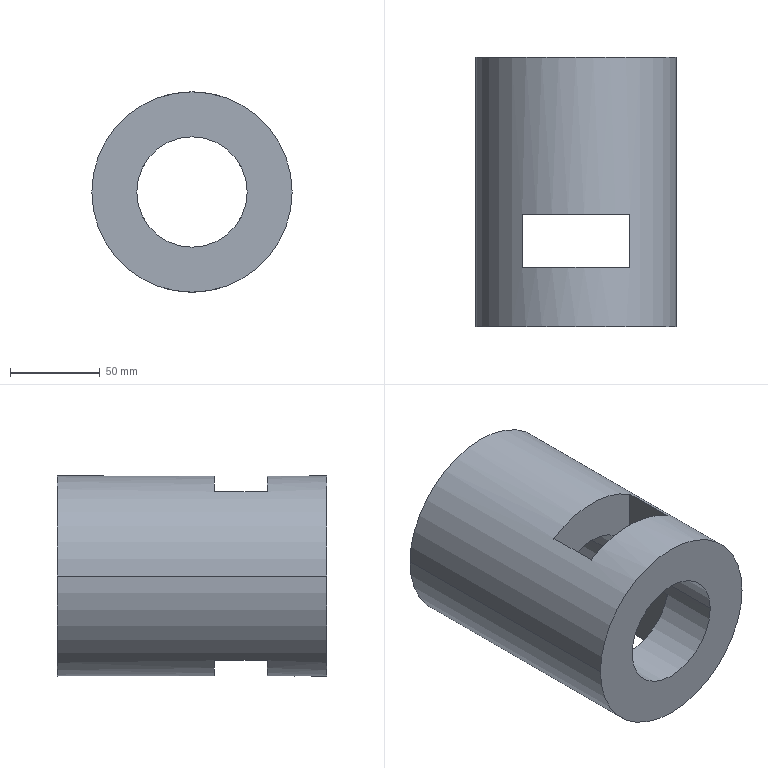Part | STEP file | Input 1-5 | 1 solid | 17 faces | box 111.5 x 150 x 111.5 mm | volume 917688 mm3 | plane 11 | cylinder 6 | commonest cylinder face diameters 10 x2 61.5 x2 111.5 x2
STEP:
#1=CARTESIAN_POINT('',(-753.859,1587.424,3132.342));
#2=VERTEX_POINT('',#1);
#3=CARTESIAN_POINT('',(-743.859,1587.424,3132.342));
#4=VERTEX_POINT('',#3);
#5=CARTESIAN_POINT('',(-748.859,1587.424,3132.342));
#6=DIRECTION('',(0.,0.,-1.));
#7=DIRECTION('',(1.,0.,0.));
#8=AXIS2_PLACEMENT_3D('',#5,#6,#7);
#9=CIRCLE('',#8,5.);
#10=EDGE_CURVE('',#2,#4,#9,.T.);
#11=ORIENTED_EDGE('',*,*,#10,.F.);
#12=CARTESIAN_POINT('',(-753.859,1587.424,3116.816));
#13=VERTEX_POINT('',#12);
#14=CARTESIAN_POINT('',(-753.859,1587.424,3132.342));
#15=DIRECTION('',(0.,0.,1.));
#16=VECTOR('',#15,1000.);
#17=LINE('',#14,#16);
#18=EDGE_CURVE('',#13,#2,#17,.T.);
#19=ORIENTED_EDGE('',*,*,#18,.F.);
#20=CARTESIAN_POINT('',(-743.859,1587.424,3116.816));
#21=VERTEX_POINT('',#20);
#22=CARTESIAN_POINT('',(-743.859,1587.424,3116.816));
#23=CARTESIAN_POINT('',(-743.859,1587.754,3116.816));
#24=CARTESIAN_POINT('',(-743.891,1588.079,3116.813));
#25=CARTESIAN_POINT('',(-743.987,1588.558,3116.805));
#26=CARTESIAN_POINT('',(-744.026,1588.717,3116.802));
#27=CARTESIAN_POINT('',(-744.121,1589.031,3116.793));
#28=CARTESIAN_POINT('',(-744.177,1589.187,3116.789));
#29=CARTESIAN_POINT('',(-744.365,1589.641,3116.773));
#30=CARTESIAN_POINT('',(-744.519,1589.928,3116.761));
#31=CARTESIAN_POINT('',(-744.882,1590.472,3116.733));
#32=CARTESIAN_POINT('',(-745.093,1590.729,3116.719));
#33=CARTESIAN_POINT('',(-745.554,1591.19,3116.689));
#34=CARTESIAN_POINT('',(-745.805,1591.397,3116.675));
#35=CARTESIAN_POINT('',(-746.352,1591.762,3116.647));
#36=CARTESIAN_POINT('',(-746.643,1591.917,3116.635));
#37=CARTESIAN_POINT('',(-747.244,1592.167,3116.614));
#38=CARTESIAN_POINT('',(-747.559,1592.263,3116.606));
#39=CARTESIAN_POINT('',(-748.205,1592.391,3116.595));
#40=CARTESIAN_POINT('',(-748.529,1592.423,3116.592));
#41=CARTESIAN_POINT('',(-749.182,1592.424,3116.592));
#42=CARTESIAN_POINT('',(-749.513,1592.391,3116.595));
#43=CARTESIAN_POINT('',(-750.154,1592.264,3116.606));
#44=CARTESIAN_POINT('',(-750.466,1592.17,3116.614));
#45=CARTESIAN_POINT('',(-750.92,1591.982,3116.63));
#46=CARTESIAN_POINT('',(-751.07,1591.911,3116.635));
#47=CARTESIAN_POINT('',(-751.36,1591.756,3116.648));
#48=CARTESIAN_POINT('',(-751.5,1591.672,3116.654));
#49=CARTESIAN_POINT('',(-751.906,1591.401,3116.674));
#50=CARTESIAN_POINT('',(-752.158,1591.195,3116.689));
#51=CARTESIAN_POINT('',(-752.625,1590.728,3116.719));
#52=CARTESIAN_POINT('',(-752.832,1590.476,3116.733));
#53=CARTESIAN_POINT('',(-753.104,1590.07,3116.754));
#54=CARTESIAN_POINT('',(-753.188,1589.93,3116.76));
#55=CARTESIAN_POINT('',(-753.343,1589.641,3116.772));
#56=CARTESIAN_POINT('',(-753.414,1589.491,3116.778));
#57=CARTESIAN_POINT('',(-753.603,1589.037,3116.794));
#58=CARTESIAN_POINT('',(-753.697,1588.726,3116.802));
#59=CARTESIAN_POINT('',(-753.826,1588.085,3116.813));
#60=CARTESIAN_POINT('',(-753.859,1587.754,3116.816));
#61=CARTESIAN_POINT('',(-753.859,1587.424,3116.816));
#62=B_SPLINE_CURVE_WITH_KNOTS('',3,(#22,#23,#24,#25,#26,#27,#28,#29,#30,#31,#32,#33,#34,#35,#36,#37,#38,#39,#40,#41,#42,#43,#44,#45,#46,#47,#48,#49,#50,#51,#52,#53,#54,#55,#56,#57,#58,#59,#60,#61),.UNSPECIFIED.,.F.,.F.,(4,2,2,2,2,2,2,2,2,2,2,2,2,2,2,2,2,2,2,4),(0.,0.0009773,0.001466,0.001955,0.002932,0.003909,0.004886,0.005864,0.006841,0.007818,0.008796,0.009773,0.01026,0.01075,0.01173,0.0127,0.01319,0.01368,0.01466,0.01564),.UNSPECIFIED.);
#63=EDGE_CURVE('',#21,#13,#62,.T.);
#64=ORIENTED_EDGE('',*,*,#63,.F.);
#65=CARTESIAN_POINT('',(-743.859,1587.424,3132.342));
#66=DIRECTION('',(0.,0.,1.));
#67=VECTOR('',#66,1000.);
#68=LINE('',#65,#67);
#69=EDGE_CURVE('',#21,#4,#68,.T.);
#70=ORIENTED_EDGE('',*,*,#69,.T.);
#71=EDGE_LOOP('',(#11,#19,#64,#70));
#72=FACE_OUTER_BOUND('',#71,.T.);
#73=CARTESIAN_POINT('',(-748.859,1587.424,3132.342));
#74=DIRECTION('',(0.,0.,-1.));
#75=DIRECTION('',(-1.,0.,0.));
#76=AXIS2_PLACEMENT_3D('',#73,#74,#75);
#77=CYLINDRICAL_SURFACE('',#76,5.);
#78=ADVANCED_FACE('',(#72),#77,.F.);
#79=CARTESIAN_POINT('',(-718.859,1636.918,3179.092));
#80=VERTEX_POINT('',#79);
#81=CARTESIAN_POINT('',(-718.859,1607.418,3179.092));
#82=VERTEX_POINT('',#81);
#83=CARTESIAN_POINT('',(-718.859,1574.418,3179.092));
#84=DIRECTION('',(0.,-1.,0.));
#85=VECTOR('',#84,1000.);
#86=LINE('',#83,#85);
#87=EDGE_CURVE('',#80,#82,#86,.T.);
#88=ORIENTED_EDGE('',*,*,#87,.F.);
#89=CARTESIAN_POINT('',(-778.859,1636.918,3179.092));
#90=VERTEX_POINT('',#89);
#91=CARTESIAN_POINT('',(-748.859,1636.918,3172.342));
#92=DIRECTION('',(0.,1.,0.));
#93=DIRECTION('',(1.,0.,0.));
#94=AXIS2_PLACEMENT_3D('',#91,#92,#93);
#95=CIRCLE('',#94,30.75);
#96=EDGE_CURVE('',#90,#80,#95,.T.);
#97=ORIENTED_EDGE('',*,*,#96,.F.);
#98=CARTESIAN_POINT('',(-778.859,1607.418,3179.092));
#99=VERTEX_POINT('',#98);
#100=CARTESIAN_POINT('',(-778.859,1574.418,3179.092));
#101=DIRECTION('',(0.,1.,0.));
#102=VECTOR('',#101,1000.);
#103=LINE('',#100,#102);
#104=EDGE_CURVE('',#99,#90,#103,.T.);
#105=ORIENTED_EDGE('',*,*,#104,.F.);
#106=CARTESIAN_POINT('',(-748.859,1607.418,3172.342));
#107=DIRECTION('',(0.,-1.,0.));
#108=DIRECTION('',(-1.,0.,0.));
#109=AXIS2_PLACEMENT_3D('',#106,#107,#108);
#110=CIRCLE('',#109,30.75);
#111=EDGE_CURVE('',#82,#99,#110,.T.);
#112=ORIENTED_EDGE('',*,*,#111,.F.);
#113=EDGE_LOOP('',(#88,#97,#105,#112));
#114=FACE_BOUND('',#113,.T.);
#115=CARTESIAN_POINT('',(-718.109,1574.418,3172.342));
#116=VERTEX_POINT('',#115);
#117=CARTESIAN_POINT('',(-779.609,1574.418,3172.342));
#118=VERTEX_POINT('',#117);
#119=CARTESIAN_POINT('',(-748.859,1574.418,3172.342));
#120=DIRECTION('',(0.,-1.,0.));
#121=DIRECTION('',(-1.,0.,0.));
#122=AXIS2_PLACEMENT_3D('',#119,#120,#121);
#123=CIRCLE('',#122,30.75);
#124=EDGE_CURVE('',#116,#118,#123,.T.);
#125=ORIENTED_EDGE('',*,*,#124,.T.);
#126=CARTESIAN_POINT('',(-779.609,1724.418,3172.342));
#127=VERTEX_POINT('',#126);
#128=CARTESIAN_POINT('',(-779.609,1574.418,3172.342));
#129=DIRECTION('',(0.,-1.,0.));
#130=VECTOR('',#129,1000.);
#131=LINE('',#128,#130);
#132=EDGE_CURVE('',#127,#118,#131,.T.);
#133=ORIENTED_EDGE('',*,*,#132,.F.);
#134=CARTESIAN_POINT('',(-718.109,1724.418,3172.342));
#135=VERTEX_POINT('',#134);
#136=CARTESIAN_POINT('',(-748.859,1724.418,3172.342));
#137=DIRECTION('',(0.,-1.,0.));
#138=DIRECTION('',(-1.,0.,0.));
#139=AXIS2_PLACEMENT_3D('',#136,#137,#138);
#140=CIRCLE('',#139,30.75);
#141=EDGE_CURVE('',#135,#127,#140,.T.);
#142=ORIENTED_EDGE('',*,*,#141,.F.);
#143=CARTESIAN_POINT('',(-718.109,1574.418,3172.342));
#144=DIRECTION('',(0.,-1.,0.));
#145=VECTOR('',#144,1000.);
#146=LINE('',#143,#145);
#147=EDGE_CURVE('',#135,#116,#146,.T.);
#148=ORIENTED_EDGE('',*,*,#147,.T.);
#149=EDGE_LOOP('',(#125,#133,#142,#148));
#150=FACE_OUTER_BOUND('',#149,.T.);
#151=CARTESIAN_POINT('',(-748.859,1574.418,3172.342));
#152=DIRECTION('',(0.,1.,0.));
#153=DIRECTION('',(-1.,0.,0.));
#154=AXIS2_PLACEMENT_3D('',#151,#152,#153);
#155=CYLINDRICAL_SURFACE('',#154,30.75);
#156=ADVANCED_FACE('',(#114,#150),#155,.F.);
#157=CARTESIAN_POINT('',(-778.859,1607.418,3125.352));
#158=VERTEX_POINT('',#157);
#159=CARTESIAN_POINT('',(-718.859,1607.418,3125.352));
#160=VERTEX_POINT('',#159);
#161=CARTESIAN_POINT('',(-748.859,1607.418,3172.342));
#162=DIRECTION('',(0.,-1.,0.));
#163=DIRECTION('',(-1.,0.,0.));
#164=AXIS2_PLACEMENT_3D('',#161,#162,#163);
#165=CIRCLE('',#164,55.75);
#166=EDGE_CURVE('',#158,#160,#165,.T.);
#167=ORIENTED_EDGE('',*,*,#166,.T.);
#168=CARTESIAN_POINT('',(-718.859,1636.918,3125.352));
#169=VERTEX_POINT('',#168);
#170=CARTESIAN_POINT('',(-718.859,1574.418,3125.352));
#171=DIRECTION('',(0.,1.,0.));
#172=VECTOR('',#171,1000.);
#173=LINE('',#170,#172);
#174=EDGE_CURVE('',#160,#169,#173,.T.);
#175=ORIENTED_EDGE('',*,*,#174,.T.);
#176=CARTESIAN_POINT('',(-778.859,1636.918,3125.352));
#177=VERTEX_POINT('',#176);
#178=CARTESIAN_POINT('',(-748.859,1636.918,3172.342));
#179=DIRECTION('',(0.,1.,0.));
#180=DIRECTION('',(1.,0.,0.));
#181=AXIS2_PLACEMENT_3D('',#178,#179,#180);
#182=CIRCLE('',#181,55.75);
#183=EDGE_CURVE('',#169,#177,#182,.T.);
#184=ORIENTED_EDGE('',*,*,#183,.T.);
#185=CARTESIAN_POINT('',(-778.859,1574.418,3125.352));
#186=DIRECTION('',(0.,-1.,0.));
#187=VECTOR('',#186,1000.);
#188=LINE('',#185,#187);
#189=EDGE_CURVE('',#177,#158,#188,.T.);
#190=ORIENTED_EDGE('',*,*,#189,.T.);
#191=EDGE_LOOP('',(#167,#175,#184,#190));
#192=FACE_BOUND('',#191,.T.);
#193=ORIENTED_EDGE('',*,*,#63,.T.);
#194=CARTESIAN_POINT('',(-753.859,1587.424,3116.816));
#195=CARTESIAN_POINT('',(-753.859,1587.093,3116.816));
#196=CARTESIAN_POINT('',(-753.826,1586.768,3116.813));
#197=CARTESIAN_POINT('',(-753.731,1586.289,3116.805));
#198=CARTESIAN_POINT('',(-753.691,1586.13,3116.802));
#199=CARTESIAN_POINT('',(-753.596,1585.816,3116.793));
#200=CARTESIAN_POINT('',(-753.54,1585.66,3116.789));
#201=CARTESIAN_POINT('',(-753.352,1585.206,3116.773));
#202=CARTESIAN_POINT('',(-753.199,1584.919,3116.761));
#203=CARTESIAN_POINT('',(-752.836,1584.376,3116.733));
#204=CARTESIAN_POINT('',(-752.625,1584.118,3116.719));
#205=CARTESIAN_POINT('',(-752.164,1583.657,3116.689));
#206=CARTESIAN_POINT('',(-751.912,1583.451,3116.675));
#207=CARTESIAN_POINT('',(-751.366,1583.085,3116.647));
#208=CARTESIAN_POINT('',(-751.075,1582.93,3116.635));
#209=CARTESIAN_POINT('',(-750.474,1582.68,3116.614));
#210=CARTESIAN_POINT('',(-750.158,1582.584,3116.606));
#211=CARTESIAN_POINT('',(-749.513,1582.456,3116.595));
#212=CARTESIAN_POINT('',(-749.189,1582.424,3116.592));
#213=CARTESIAN_POINT('',(-748.536,1582.423,3116.592));
#214=CARTESIAN_POINT('',(-748.205,1582.456,3116.595));
#215=CARTESIAN_POINT('',(-747.563,1582.583,3116.606));
#216=CARTESIAN_POINT('',(-747.252,1582.678,3116.614));
#217=CARTESIAN_POINT('',(-746.797,1582.865,3116.63));
#218=CARTESIAN_POINT('',(-746.648,1582.936,3116.635));
#219=CARTESIAN_POINT('',(-746.358,1583.091,3116.648));
#220=CARTESIAN_POINT('',(-746.218,1583.175,3116.654));
#221=CARTESIAN_POINT('',(-745.812,1583.446,3116.674));
#222=CARTESIAN_POINT('',(-745.559,1583.652,3116.689));
#223=CARTESIAN_POINT('',(-745.092,1584.119,3116.719));
#224=CARTESIAN_POINT('',(-744.885,1584.371,3116.733));
#225=CARTESIAN_POINT('',(-744.613,1584.777,3116.754));
#226=CARTESIAN_POINT('',(-744.529,1584.917,3116.76));
#227=CARTESIAN_POINT('',(-744.374,1585.206,3116.772));
#228=CARTESIAN_POINT('',(-744.303,1585.356,3116.778));
#229=CARTESIAN_POINT('',(-744.115,1585.81,3116.794));
#230=CARTESIAN_POINT('',(-744.02,1586.122,3116.802));
#231=CARTESIAN_POINT('',(-743.892,1586.762,3116.813));
#232=CARTESIAN_POINT('',(-743.859,1587.093,3116.816));
#233=CARTESIAN_POINT('',(-743.859,1587.424,3116.816));
#234=B_SPLINE_CURVE_WITH_KNOTS('',3,(#194,#195,#196,#197,#198,#199,#200,#201,#202,#203,#204,#205,#206,#207,#208,#209,#210,#211,#212,#213,#214,#215,#216,#217,#218,#219,#220,#221,#222,#223,#224,#225,#226,#227,#228,#229,#230,#231,#232,#233),.UNSPECIFIED.,.F.,.F.,(4,2,2,2,2,2,2,2,2,2,2,2,2,2,2,2,2,2,2,4),(0.,0.0009773,0.001466,0.001955,0.002932,0.003909,0.004886,0.005864,0.006841,0.007818,0.008796,0.009773,0.01026,0.01075,0.01173,0.0127,0.01319,0.01368,0.01466,0.01564),.UNSPECIFIED.);
#235=EDGE_CURVE('',#13,#21,#234,.T.);
#236=ORIENTED_EDGE('',*,*,#235,.T.);
#237=EDGE_LOOP('',(#193,#236));
#238=FACE_BOUND('',#237,.T.);
#239=CARTESIAN_POINT('',(-804.609,1574.418,3172.342));
#240=VERTEX_POINT('',#239);
#241=CARTESIAN_POINT('',(-693.109,1574.418,3172.342));
#242=VERTEX_POINT('',#241);
#243=CARTESIAN_POINT('',(-748.859,1574.418,3172.342));
#244=DIRECTION('',(0.,-1.,0.));
#245=DIRECTION('',(-1.,0.,0.));
#246=AXIS2_PLACEMENT_3D('',#243,#244,#245);
#247=CIRCLE('',#246,55.75);
#248=EDGE_CURVE('',#240,#242,#247,.T.);
#249=ORIENTED_EDGE('',*,*,#248,.F.);
#250=CARTESIAN_POINT('',(-804.609,1724.418,3172.342));
#251=VERTEX_POINT('',#250);
#252=CARTESIAN_POINT('',(-804.609,1574.418,3172.342));
#253=DIRECTION('',(0.,-1.,0.));
#254=VECTOR('',#253,1000.);
#255=LINE('',#252,#254);
#256=EDGE_CURVE('',#251,#240,#255,.T.);
#257=ORIENTED_EDGE('',*,*,#256,.F.);
#258=CARTESIAN_POINT('',(-693.109,1724.418,3172.342));
#259=VERTEX_POINT('',#258);
#260=CARTESIAN_POINT('',(-748.859,1724.418,3172.342));
#261=DIRECTION('',(0.,-1.,0.));
#262=DIRECTION('',(-1.,0.,0.));
#263=AXIS2_PLACEMENT_3D('',#260,#261,#262);
#264=CIRCLE('',#263,55.75);
#265=EDGE_CURVE('',#251,#259,#264,.T.);
#266=ORIENTED_EDGE('',*,*,#265,.T.);
#267=CARTESIAN_POINT('',(-693.109,1574.418,3172.342));
#268=DIRECTION('',(0.,-1.,0.));
#269=VECTOR('',#268,1000.);
#270=LINE('',#267,#269);
#271=EDGE_CURVE('',#259,#242,#270,.T.);
#272=ORIENTED_EDGE('',*,*,#271,.T.);
#273=EDGE_LOOP('',(#249,#257,#266,#272));
#274=FACE_OUTER_BOUND('',#273,.T.);
#275=CARTESIAN_POINT('',(-748.859,1574.418,3172.342));
#276=DIRECTION('',(0.,1.,0.));
#277=DIRECTION('',(-1.,0.,0.));
#278=AXIS2_PLACEMENT_3D('',#275,#276,#277);
#279=CYLINDRICAL_SURFACE('',#278,55.75);
#280=ADVANCED_FACE('',(#192,#238,#274),#279,.T.);
#281=CARTESIAN_POINT('',(-748.859,1574.418,3172.342));
#282=DIRECTION('',(0.,-1.,0.));
#283=DIRECTION('',(-1.,0.,0.));
#284=AXIS2_PLACEMENT_3D('',#281,#282,#283);
#285=CIRCLE('',#284,55.75);
#286=EDGE_CURVE('',#242,#240,#285,.T.);
#287=ORIENTED_EDGE('',*,*,#286,.T.);
#288=ORIENTED_EDGE('',*,*,#248,.T.);
#289=EDGE_LOOP('',(#287,#288));
#290=FACE_OUTER_BOUND('',#289,.T.);
#291=ORIENTED_EDGE('',*,*,#124,.F.);
#292=CARTESIAN_POINT('',(-748.859,1574.418,3172.342));
#293=DIRECTION('',(0.,-1.,0.));
#294=DIRECTION('',(-1.,0.,0.));
#295=AXIS2_PLACEMENT_3D('',#292,#293,#294);
#296=CIRCLE('',#295,30.75);
#297=EDGE_CURVE('',#118,#116,#296,.T.);
#298=ORIENTED_EDGE('',*,*,#297,.F.);
#299=EDGE_LOOP('',(#291,#298));
#300=FACE_BOUND('',#299,.T.);
#301=CARTESIAN_POINT('',(-748.859,1574.418,3172.342));
#302=DIRECTION('',(0.,-1.,0.));
#303=DIRECTION('',(1.,0.,0.));
#304=AXIS2_PLACEMENT_3D('',#301,#302,#303);
#305=PLANE('',#304);
#306=ADVANCED_FACE('',(#290,#300),#305,.T.);
#307=CARTESIAN_POINT('',(-748.859,1724.418,3172.342));
#308=DIRECTION('',(0.,-1.,0.));
#309=DIRECTION('',(-1.,0.,0.));
#310=AXIS2_PLACEMENT_3D('',#307,#308,#309);
#311=CIRCLE('',#310,55.75);
#312=EDGE_CURVE('',#259,#251,#311,.T.);
#313=ORIENTED_EDGE('',*,*,#312,.F.);
#314=ORIENTED_EDGE('',*,*,#265,.F.);
#315=EDGE_LOOP('',(#313,#314));
#316=FACE_OUTER_BOUND('',#315,.T.);
#317=ORIENTED_EDGE('',*,*,#141,.T.);
#318=CARTESIAN_POINT('',(-748.859,1724.418,3172.342));
#319=DIRECTION('',(0.,-1.,0.));
#320=DIRECTION('',(-1.,0.,0.));
#321=AXIS2_PLACEMENT_3D('',#318,#319,#320);
#322=CIRCLE('',#321,30.75);
#323=EDGE_CURVE('',#127,#135,#322,.T.);
#324=ORIENTED_EDGE('',*,*,#323,.T.);
#325=EDGE_LOOP('',(#317,#324));
#326=FACE_BOUND('',#325,.T.);
#327=CARTESIAN_POINT('',(-748.859,1724.418,3172.342));
#328=DIRECTION('',(0.,-1.,0.));
#329=DIRECTION('',(1.,0.,0.));
#330=AXIS2_PLACEMENT_3D('',#327,#328,#329);
#331=PLANE('',#330);
#332=ADVANCED_FACE('',(#316,#326),#331,.F.);
#333=ORIENTED_EDGE('',*,*,#256,.T.);
#334=ORIENTED_EDGE('',*,*,#286,.F.);
#335=ORIENTED_EDGE('',*,*,#271,.F.);
#336=ORIENTED_EDGE('',*,*,#312,.T.);
#337=EDGE_LOOP('',(#333,#334,#335,#336));
#338=FACE_OUTER_BOUND('',#337,.T.);
#339=CARTESIAN_POINT('',(-778.859,1636.918,3219.332));
#340=VERTEX_POINT('',#339);
#341=CARTESIAN_POINT('',(-718.859,1636.918,3219.332));
#342=VERTEX_POINT('',#341);
#343=CARTESIAN_POINT('',(-748.859,1636.918,3172.342));
#344=DIRECTION('',(0.,1.,0.));
#345=DIRECTION('',(1.,0.,0.));
#346=AXIS2_PLACEMENT_3D('',#343,#344,#345);
#347=CIRCLE('',#346,55.75);
#348=EDGE_CURVE('',#340,#342,#347,.T.);
#349=ORIENTED_EDGE('',*,*,#348,.T.);
#350=CARTESIAN_POINT('',(-718.859,1607.418,3219.332));
#351=VERTEX_POINT('',#350);
#352=CARTESIAN_POINT('',(-718.859,1574.418,3219.332));
#353=DIRECTION('',(0.,-1.,0.));
#354=VECTOR('',#353,1000.);
#355=LINE('',#352,#354);
#356=EDGE_CURVE('',#342,#351,#355,.T.);
#357=ORIENTED_EDGE('',*,*,#356,.T.);
#358=CARTESIAN_POINT('',(-778.859,1607.418,3219.332));
#359=VERTEX_POINT('',#358);
#360=CARTESIAN_POINT('',(-748.859,1607.418,3172.342));
#361=DIRECTION('',(0.,-1.,0.));
#362=DIRECTION('',(-1.,0.,0.));
#363=AXIS2_PLACEMENT_3D('',#360,#361,#362);
#364=CIRCLE('',#363,55.75);
#365=EDGE_CURVE('',#351,#359,#364,.T.);
#366=ORIENTED_EDGE('',*,*,#365,.T.);
#367=CARTESIAN_POINT('',(-778.859,1574.418,3219.332));
#368=DIRECTION('',(0.,1.,0.));
#369=VECTOR('',#368,1000.);
#370=LINE('',#367,#369);
#371=EDGE_CURVE('',#359,#340,#370,.T.);
#372=ORIENTED_EDGE('',*,*,#371,.T.);
#373=EDGE_LOOP('',(#349,#357,#366,#372));
#374=FACE_BOUND('',#373,.T.);
#375=CARTESIAN_POINT('',(-748.859,1574.418,3172.342));
#376=DIRECTION('',(0.,1.,0.));
#377=DIRECTION('',(-1.,0.,0.));
#378=AXIS2_PLACEMENT_3D('',#375,#376,#377);
#379=CYLINDRICAL_SURFACE('',#378,55.75);
#380=ADVANCED_FACE('',(#338,#374),#379,.T.);
#381=ORIENTED_EDGE('',*,*,#132,.T.);
#382=ORIENTED_EDGE('',*,*,#297,.T.);
#383=ORIENTED_EDGE('',*,*,#147,.F.);
#384=ORIENTED_EDGE('',*,*,#323,.F.);
#385=EDGE_LOOP('',(#381,#382,#383,#384));
#386=FACE_OUTER_BOUND('',#385,.T.);
#387=CARTESIAN_POINT('',(-718.859,1607.418,3165.592));
#388=VERTEX_POINT('',#387);
#389=CARTESIAN_POINT('',(-718.859,1636.918,3165.592));
#390=VERTEX_POINT('',#389);
#391=CARTESIAN_POINT('',(-718.859,1574.418,3165.592));
#392=DIRECTION('',(0.,1.,0.));
#393=VECTOR('',#392,1000.);
#394=LINE('',#391,#393);
#395=EDGE_CURVE('',#388,#390,#394,.T.);
#396=ORIENTED_EDGE('',*,*,#395,.F.);
#397=CARTESIAN_POINT('',(-778.859,1607.418,3165.592));
#398=VERTEX_POINT('',#397);
#399=CARTESIAN_POINT('',(-748.859,1607.418,3172.342));
#400=DIRECTION('',(0.,-1.,0.));
#401=DIRECTION('',(-1.,0.,0.));
#402=AXIS2_PLACEMENT_3D('',#399,#400,#401);
#403=CIRCLE('',#402,30.75);
#404=EDGE_CURVE('',#398,#388,#403,.T.);
#405=ORIENTED_EDGE('',*,*,#404,.F.);
#406=CARTESIAN_POINT('',(-778.859,1636.918,3165.592));
#407=VERTEX_POINT('',#406);
#408=CARTESIAN_POINT('',(-778.859,1574.418,3165.592));
#409=DIRECTION('',(0.,-1.,0.));
#410=VECTOR('',#409,1000.);
#411=LINE('',#408,#410);
#412=EDGE_CURVE('',#407,#398,#411,.T.);
#413=ORIENTED_EDGE('',*,*,#412,.F.);
#414=CARTESIAN_POINT('',(-748.859,1636.918,3172.342));
#415=DIRECTION('',(0.,1.,0.));
#416=DIRECTION('',(1.,0.,0.));
#417=AXIS2_PLACEMENT_3D('',#414,#415,#416);
#418=CIRCLE('',#417,30.75);
#419=EDGE_CURVE('',#390,#407,#418,.T.);
#420=ORIENTED_EDGE('',*,*,#419,.F.);
#421=EDGE_LOOP('',(#396,#405,#413,#420));
#422=FACE_BOUND('',#421,.T.);
#423=CARTESIAN_POINT('',(-748.859,1574.418,3172.342));
#424=DIRECTION('',(0.,1.,0.));
#425=DIRECTION('',(-1.,0.,0.));
#426=AXIS2_PLACEMENT_3D('',#423,#424,#425);
#427=CYLINDRICAL_SURFACE('',#426,30.75);
#428=ADVANCED_FACE('',(#386,#422),#427,.F.);
#429=CARTESIAN_POINT('',(-718.859,1607.418,3252.342));
#430=DIRECTION('',(0.,0.,-1.));
#431=VECTOR('',#430,1000.);
#432=LINE('',#429,#431);
#433=EDGE_CURVE('',#351,#82,#432,.T.);
#434=ORIENTED_EDGE('',*,*,#433,.T.);
#435=ORIENTED_EDGE('',*,*,#111,.T.);
#436=CARTESIAN_POINT('',(-778.859,1607.418,3252.342));
#437=DIRECTION('',(0.,0.,-1.));
#438=VECTOR('',#437,1000.);
#439=LINE('',#436,#438);
#440=EDGE_CURVE('',#359,#99,#439,.T.);
#441=ORIENTED_EDGE('',*,*,#440,.F.);
#442=ORIENTED_EDGE('',*,*,#365,.F.);
#443=EDGE_LOOP('',(#434,#435,#441,#442));
#444=FACE_OUTER_BOUND('',#443,.T.);
#445=CARTESIAN_POINT('',(-778.859,1607.418,3252.342));
#446=DIRECTION('',(0.,-1.,0.));
#447=DIRECTION('',(1.,0.,0.));
#448=AXIS2_PLACEMENT_3D('',#445,#446,#447);
#449=PLANE('',#448);
#450=ADVANCED_FACE('',(#444),#449,.F.);
#451=ORIENTED_EDGE('',*,*,#440,.T.);
#452=ORIENTED_EDGE('',*,*,#104,.T.);
#453=CARTESIAN_POINT('',(-778.859,1636.918,3252.342));
#454=DIRECTION('',(0.,0.,-1.));
#455=VECTOR('',#454,1000.);
#456=LINE('',#453,#455);
#457=EDGE_CURVE('',#340,#90,#456,.T.);
#458=ORIENTED_EDGE('',*,*,#457,.F.);
#459=ORIENTED_EDGE('',*,*,#371,.F.);
#460=EDGE_LOOP('',(#451,#452,#458,#459));
#461=FACE_OUTER_BOUND('',#460,.T.);
#462=CARTESIAN_POINT('',(-778.859,1636.918,3252.342));
#463=DIRECTION('',(-1.,0.,0.));
#464=DIRECTION('',(0.,0.,1.));
#465=AXIS2_PLACEMENT_3D('',#462,#463,#464);
#466=PLANE('',#465);
#467=ADVANCED_FACE('',(#461),#466,.F.);
#468=ORIENTED_EDGE('',*,*,#457,.T.);
#469=ORIENTED_EDGE('',*,*,#96,.T.);
#470=CARTESIAN_POINT('',(-718.859,1636.918,3252.342));
#471=DIRECTION('',(0.,0.,-1.));
#472=VECTOR('',#471,1000.);
#473=LINE('',#470,#472);
#474=EDGE_CURVE('',#342,#80,#473,.T.);
#475=ORIENTED_EDGE('',*,*,#474,.F.);
#476=ORIENTED_EDGE('',*,*,#348,.F.);
#477=EDGE_LOOP('',(#468,#469,#475,#476));
#478=FACE_OUTER_BOUND('',#477,.T.);
#479=CARTESIAN_POINT('',(-778.859,1636.918,3252.342));
#480=DIRECTION('',(0.,1.,0.));
#481=DIRECTION('',(-1.,0.,0.));
#482=AXIS2_PLACEMENT_3D('',#479,#480,#481);
#483=PLANE('',#482);
#484=ADVANCED_FACE('',(#478),#483,.F.);
#485=ORIENTED_EDGE('',*,*,#474,.T.);
#486=ORIENTED_EDGE('',*,*,#87,.T.);
#487=ORIENTED_EDGE('',*,*,#433,.F.);
#488=ORIENTED_EDGE('',*,*,#356,.F.);
#489=EDGE_LOOP('',(#485,#486,#487,#488));
#490=FACE_OUTER_BOUND('',#489,.T.);
#491=CARTESIAN_POINT('',(-718.859,1636.918,3252.342));
#492=DIRECTION('',(1.,0.,0.));
#493=DIRECTION('',(0.,0.,-1.));
#494=AXIS2_PLACEMENT_3D('',#491,#492,#493);
#495=PLANE('',#494);
#496=ADVANCED_FACE('',(#490),#495,.F.);
#497=CARTESIAN_POINT('',(-718.859,1607.418,3252.342));
#498=DIRECTION('',(0.,0.,-1.));
#499=VECTOR('',#498,1000.);
#500=LINE('',#497,#499);
#501=EDGE_CURVE('',#388,#160,#500,.T.);
#502=ORIENTED_EDGE('',*,*,#501,.F.);
#503=ORIENTED_EDGE('',*,*,#395,.T.);
#504=CARTESIAN_POINT('',(-718.859,1636.918,3252.342));
#505=DIRECTION('',(0.,0.,-1.));
#506=VECTOR('',#505,1000.);
#507=LINE('',#504,#506);
#508=EDGE_CURVE('',#390,#169,#507,.T.);
#509=ORIENTED_EDGE('',*,*,#508,.T.);
#510=ORIENTED_EDGE('',*,*,#174,.F.);
#511=EDGE_LOOP('',(#502,#503,#509,#510));
#512=FACE_OUTER_BOUND('',#511,.T.);
#513=CARTESIAN_POINT('',(-718.859,1636.918,3252.342));
#514=DIRECTION('',(1.,0.,0.));
#515=DIRECTION('',(0.,0.,-1.));
#516=AXIS2_PLACEMENT_3D('',#513,#514,#515);
#517=PLANE('',#516);
#518=ADVANCED_FACE('',(#512),#517,.F.);
#519=ORIENTED_EDGE('',*,*,#508,.F.);
#520=ORIENTED_EDGE('',*,*,#419,.T.);
#521=CARTESIAN_POINT('',(-778.859,1636.918,3252.342));
#522=DIRECTION('',(0.,0.,-1.));
#523=VECTOR('',#522,1000.);
#524=LINE('',#521,#523);
#525=EDGE_CURVE('',#407,#177,#524,.T.);
#526=ORIENTED_EDGE('',*,*,#525,.T.);
#527=ORIENTED_EDGE('',*,*,#183,.F.);
#528=EDGE_LOOP('',(#519,#520,#526,#527));
#529=FACE_OUTER_BOUND('',#528,.T.);
#530=CARTESIAN_POINT('',(-778.859,1636.918,3252.342));
#531=DIRECTION('',(0.,1.,0.));
#532=DIRECTION('',(-1.,0.,0.));
#533=AXIS2_PLACEMENT_3D('',#530,#531,#532);
#534=PLANE('',#533);
#535=ADVANCED_FACE('',(#529),#534,.F.);
#536=ORIENTED_EDGE('',*,*,#525,.F.);
#537=ORIENTED_EDGE('',*,*,#412,.T.);
#538=CARTESIAN_POINT('',(-778.859,1607.418,3252.342));
#539=DIRECTION('',(0.,0.,-1.));
#540=VECTOR('',#539,1000.);
#541=LINE('',#538,#540);
#542=EDGE_CURVE('',#398,#158,#541,.T.);
#543=ORIENTED_EDGE('',*,*,#542,.T.);
#544=ORIENTED_EDGE('',*,*,#189,.F.);
#545=EDGE_LOOP('',(#536,#537,#543,#544));
#546=FACE_OUTER_BOUND('',#545,.T.);
#547=CARTESIAN_POINT('',(-778.859,1636.918,3252.342));
#548=DIRECTION('',(-1.,0.,0.));
#549=DIRECTION('',(0.,0.,1.));
#550=AXIS2_PLACEMENT_3D('',#547,#548,#549);
#551=PLANE('',#550);
#552=ADVANCED_FACE('',(#546),#551,.F.);
#553=ORIENTED_EDGE('',*,*,#542,.F.);
#554=ORIENTED_EDGE('',*,*,#404,.T.);
#555=ORIENTED_EDGE('',*,*,#501,.T.);
#556=ORIENTED_EDGE('',*,*,#166,.F.);
#557=EDGE_LOOP('',(#553,#554,#555,#556));
#558=FACE_OUTER_BOUND('',#557,.T.);
#559=CARTESIAN_POINT('',(-778.859,1607.418,3252.342));
#560=DIRECTION('',(0.,-1.,0.));
#561=DIRECTION('',(1.,0.,0.));
#562=AXIS2_PLACEMENT_3D('',#559,#560,#561);
#563=PLANE('',#562);
#564=ADVANCED_FACE('',(#558),#563,.F.);
#565=ORIENTED_EDGE('',*,*,#18,.T.);
#566=CARTESIAN_POINT('',(-748.859,1587.424,3132.342));
#567=DIRECTION('',(0.,0.,-1.));
#568=DIRECTION('',(1.,0.,0.));
#569=AXIS2_PLACEMENT_3D('',#566,#567,#568);
#570=CIRCLE('',#569,5.);
#571=EDGE_CURVE('',#4,#2,#570,.T.);
#572=ORIENTED_EDGE('',*,*,#571,.F.);
#573=ORIENTED_EDGE('',*,*,#69,.F.);
#574=ORIENTED_EDGE('',*,*,#235,.F.);
#575=EDGE_LOOP('',(#565,#572,#573,#574));
#576=FACE_OUTER_BOUND('',#575,.T.);
#577=CARTESIAN_POINT('',(-748.859,1587.424,3132.342));
#578=DIRECTION('',(0.,0.,-1.));
#579=DIRECTION('',(-1.,0.,0.));
#580=AXIS2_PLACEMENT_3D('',#577,#578,#579);
#581=CYLINDRICAL_SURFACE('',#580,5.);
#582=ADVANCED_FACE('',(#576),#581,.F.);
#583=ORIENTED_EDGE('',*,*,#571,.T.);
#584=ORIENTED_EDGE('',*,*,#10,.T.);
#585=EDGE_LOOP('',(#583,#584));
#586=FACE_OUTER_BOUND('',#585,.T.);
#587=CARTESIAN_POINT('',(-748.859,1587.424,3132.342));
#588=DIRECTION('',(0.,0.,-1.));
#589=DIRECTION('',(-1.,0.,0.));
#590=AXIS2_PLACEMENT_3D('',#587,#588,#589);
#591=PLANE('',#590);
#592=ADVANCED_FACE('',(#586),#591,.T.);
#593=CLOSED_SHELL('',(#78,#156,#280,#306,#332,#380,#428,#450,#467,#484,#496,#518,#535,#552,#564,#582,#592));
#594=MANIFOLD_SOLID_BREP('',#593);
#595=CARTESIAN_POINT('',(0.,0.,0.));
#596=DIRECTION('',(0.,0.,1.));
#597=DIRECTION('',(1.,0.,0.));
#598=AXIS2_PLACEMENT_3D('',#595,#596,#597);
#599=(LENGTH_UNIT()NAMED_UNIT(*)SI_UNIT(.MILLI.,.METRE.));
#600=UNCERTAINTY_MEASURE_WITH_UNIT(LENGTH_MEASURE(0.00001),#599,'','');
#601=(NAMED_UNIT(*)PLANE_ANGLE_UNIT()SI_UNIT($,.RADIAN.));
#602=(NAMED_UNIT(*)SI_UNIT($,.STERADIAN.)SOLID_ANGLE_UNIT());
#603=(GEOMETRIC_REPRESENTATION_CONTEXT(3)GLOBAL_UNCERTAINTY_ASSIGNED_CONTEXT((#600))GLOBAL_UNIT_ASSIGNED_CONTEXT((#599,#601,#602))REPRESENTATION_CONTEXT('',''));
#604=ADVANCED_BREP_SHAPE_REPRESENTATION('',(#594,#598),#603);